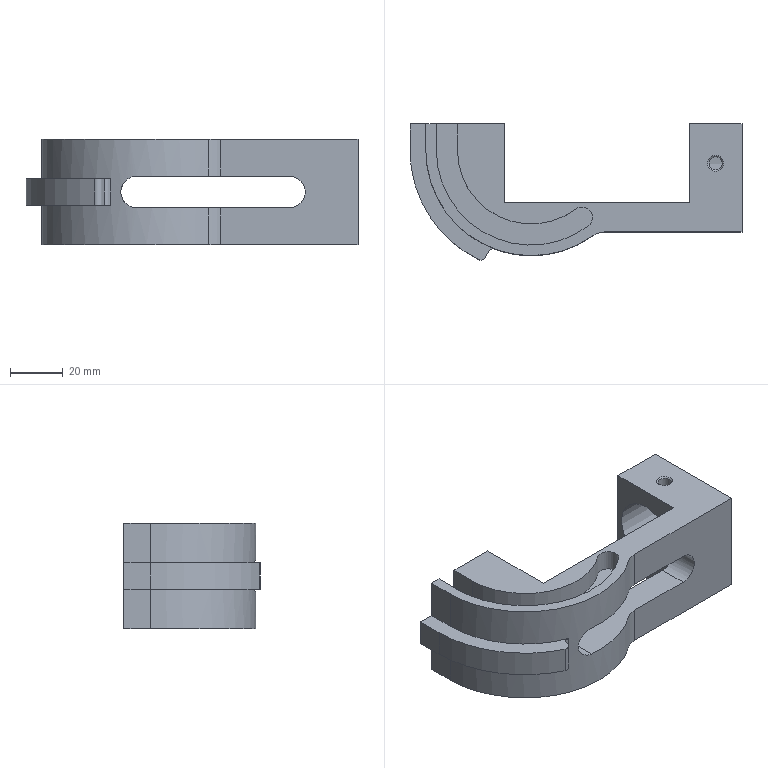Part | NX | features DATUM_CSYS 8, EXTRUDE 7, SKETCH 7, CPROJ 3, BLEND 2, EXTRACT_FACE 2, EXTRACT_STRING 2, HOLE PACKAGE 1, Instance Feature 1, Mirror Feature 1, SIMPLE HOLE 1, SYMBOLIC_THREAD 1 | 1 solid | 41 faces | box 126 x 51.679 x 40 mm | volume 90129 mm3 | plane 24 | cylinder 16 | cone 1 | commonest cylinder face diameters 4 x2 8 x2 12 x2 16 x2 56 x2 72 x2
STEP:
#1=CARTESIAN_POINT('',(-4.,-20.,-6.));
#2=VERTEX_POINT('',#1);
#3=CARTESIAN_POINT('',(-10.,-20.,0.));
#4=VERTEX_POINT('',#3);
#5=CARTESIAN_POINT('',(-4.,-20.,0.));
#6=DIRECTION('',(0.,1.,0.));
#7=DIRECTION('',(1.,0.,0.));
#8=AXIS2_PLACEMENT_3D('',#5,#6,#7);
#9=CIRCLE('',#8,6.);
#10=EDGE_CURVE('',#2,#4,#9,.T.);
#11=ORIENTED_EDGE('',*,*,#10,.F.);
#12=CARTESIAN_POINT('',(54.,-20.,-6.));
#13=VERTEX_POINT('',#12);
#14=CARTESIAN_POINT('',(54.,-20.,-6.));
#15=DIRECTION('',(-1.,0.,0.));
#16=VECTOR('',#15,1000.);
#17=LINE('',#14,#16);
#18=EDGE_CURVE('',#13,#2,#17,.T.);
#19=ORIENTED_EDGE('',*,*,#18,.F.);
#20=CARTESIAN_POINT('',(60.,-20.,0.));
#21=VERTEX_POINT('',#20);
#22=CARTESIAN_POINT('',(54.,-20.,0.));
#23=DIRECTION('',(0.,1.,0.));
#24=DIRECTION('',(1.,0.,0.));
#25=AXIS2_PLACEMENT_3D('',#22,#23,#24);
#26=CIRCLE('',#25,6.);
#27=EDGE_CURVE('',#21,#13,#26,.T.);
#28=ORIENTED_EDGE('',*,*,#27,.F.);
#29=CARTESIAN_POINT('',(60.,-20.,-20.));
#30=VERTEX_POINT('',#29);
#31=CARTESIAN_POINT('',(60.,-20.,45.));
#32=DIRECTION('',(0.,0.,-1.));
#33=VECTOR('',#32,1000.);
#34=LINE('',#31,#33);
#35=EDGE_CURVE('',#30,#21,#34,.F.);
#36=ORIENTED_EDGE('',*,*,#35,.F.);
#37=CARTESIAN_POINT('',(-10.,-20.,-20.));
#38=VERTEX_POINT('',#37);
#39=CARTESIAN_POINT('',(0.,-20.,-20.));
#40=DIRECTION('',(-1.,0.,0.));
#41=VECTOR('',#40,1000.);
#42=LINE('',#39,#41);
#43=EDGE_CURVE('',#30,#38,#42,.T.);
#44=ORIENTED_EDGE('',*,*,#43,.T.);
#45=CARTESIAN_POINT('',(-10.,-20.,45.));
#46=DIRECTION('',(0.,0.,-1.));
#47=VECTOR('',#46,1000.);
#48=LINE('',#45,#47);
#49=EDGE_CURVE('',#38,#4,#48,.F.);
#50=ORIENTED_EDGE('',*,*,#49,.T.);
#51=EDGE_LOOP('',(#11,#19,#28,#36,#44,#50));
#52=FACE_BOUND('',#51,.T.);
#53=CARTESIAN_POINT('',(-10.,-20.,45.));
#54=DIRECTION('',(0.,1.,0.));
#55=DIRECTION('',(0.,0.,1.));
#56=AXIS2_PLACEMENT_3D('',#53,#54,#55);
#57=PLANE('',#56);
#58=ADVANCED_FACE('',(#52),#57,.T.);
#59=CARTESIAN_POINT('',(23.318,-32.5,6.));
#60=VERTEX_POINT('',#59);
#61=CARTESIAN_POINT('',(23.318,-32.5,20.));
#62=VERTEX_POINT('',#61);
#63=CARTESIAN_POINT('',(23.318,-32.5,20.));
#64=DIRECTION('',(0.,0.,-1.));
#65=VECTOR('',#64,1000.);
#66=LINE('',#63,#65);
#67=EDGE_CURVE('',#60,#62,#66,.F.);
#68=ORIENTED_EDGE('',*,*,#67,.F.);
#69=CARTESIAN_POINT('',(27.982,-31.,6.));
#70=VERTEX_POINT('',#69);
#71=CARTESIAN_POINT('',(27.982,-39.,6.));
#72=DIRECTION('',(0.,0.,1.));
#73=DIRECTION('',(1.,0.,0.));
#74=AXIS2_PLACEMENT_3D('',#71,#72,#73);
#75=CIRCLE('',#74,8.);
#76=EDGE_CURVE('',#60,#70,#75,.F.);
#77=ORIENTED_EDGE('',*,*,#76,.T.);
#78=CARTESIAN_POINT('',(27.982,-31.,20.));
#79=VERTEX_POINT('',#78);
#80=CARTESIAN_POINT('',(27.982,-31.,-20.));
#81=DIRECTION('',(0.,0.,1.));
#82=VECTOR('',#81,1000.);
#83=LINE('',#80,#82);
#84=EDGE_CURVE('',#79,#70,#83,.F.);
#85=ORIENTED_EDGE('',*,*,#84,.F.);
#86=CARTESIAN_POINT('',(27.982,-39.,20.));
#87=DIRECTION('',(0.,0.,1.));
#88=DIRECTION('',(1.,0.,0.));
#89=AXIS2_PLACEMENT_3D('',#86,#87,#88);
#90=CIRCLE('',#89,8.);
#91=EDGE_CURVE('',#62,#79,#90,.F.);
#92=ORIENTED_EDGE('',*,*,#91,.F.);
#93=EDGE_LOOP('',(#68,#77,#85,#92));
#94=FACE_BOUND('',#93,.T.);
#95=CARTESIAN_POINT('',(27.982,-39.,20.));
#96=DIRECTION('',(0.,0.,-1.));
#97=DIRECTION('',(-1.,0.,0.));
#98=AXIS2_PLACEMENT_3D('',#95,#96,#97);
#99=CYLINDRICAL_SURFACE('',#98,8.);
#100=ADVANCED_FACE('',(#94),#99,.F.);
#101=CARTESIAN_POINT('',(-40.,0.,5.));
#102=VERTEX_POINT('',#101);
#103=CARTESIAN_POINT('',(-40.,10.,5.));
#104=VERTEX_POINT('',#103);
#105=CARTESIAN_POINT('',(-40.,0.,5.));
#106=DIRECTION('',(0.,1.,0.));
#107=VECTOR('',#106,1000.);
#108=LINE('',#105,#107);
#109=EDGE_CURVE('',#102,#104,#108,.T.);
#110=ORIENTED_EDGE('',*,*,#109,.F.);
#111=CARTESIAN_POINT('',(-40.,0.,20.));
#112=VERTEX_POINT('',#111);
#113=CARTESIAN_POINT('',(-40.,0.,20.));
#114=DIRECTION('',(0.,0.,-1.));
#115=VECTOR('',#114,1000.);
#116=LINE('',#113,#115);
#117=EDGE_CURVE('',#112,#102,#116,.T.);
#118=ORIENTED_EDGE('',*,*,#117,.F.);
#119=CARTESIAN_POINT('',(-40.,10.,20.));
#120=VERTEX_POINT('',#119);
#121=CARTESIAN_POINT('',(-40.,10.,20.));
#122=DIRECTION('',(0.,-1.,0.));
#123=VECTOR('',#122,1000.);
#124=LINE('',#121,#123);
#125=EDGE_CURVE('',#120,#112,#124,.T.);
#126=ORIENTED_EDGE('',*,*,#125,.F.);
#127=CARTESIAN_POINT('',(-40.,10.,20.));
#128=DIRECTION('',(0.,0.,-1.));
#129=VECTOR('',#128,1000.);
#130=LINE('',#127,#129);
#131=EDGE_CURVE('',#120,#104,#130,.T.);
#132=ORIENTED_EDGE('',*,*,#131,.T.);
#133=EDGE_LOOP('',(#110,#118,#126,#132));
#134=FACE_BOUND('',#133,.T.);
#135=CARTESIAN_POINT('',(-40.,10.,20.));
#136=DIRECTION('',(1.,0.,0.));
#137=DIRECTION('',(0.,0.,-1.));
#138=AXIS2_PLACEMENT_3D('',#135,#136,#137);
#139=PLANE('',#138);
#140=ADVANCED_FACE('',(#134),#139,.F.);
#141=CARTESIAN_POINT('',(73.,-5.,20.));
#142=VERTEX_POINT('',#141);
#143=CARTESIAN_POINT('',(70.,-5.,20.));
#144=DIRECTION('',(0.,0.,1.));
#145=DIRECTION('',(1.,0.,0.));
#146=AXIS2_PLACEMENT_3D('',#143,#144,#145);
#147=CIRCLE('',#146,3.);
#148=EDGE_CURVE('',#142,#142,#147,.F.);
#149=ORIENTED_EDGE('',*,*,#148,.T.);
#150=EDGE_LOOP('',(#149));
#151=FACE_BOUND('',#150,.T.);
#152=CARTESIAN_POINT('',(-36.,10.,20.));
#153=VERTEX_POINT('',#152);
#154=CARTESIAN_POINT('',(-36.,0.,20.));
#155=VERTEX_POINT('',#154);
#156=CARTESIAN_POINT('',(-36.,10.,20.));
#157=DIRECTION('',(0.,-1.,0.));
#158=VECTOR('',#157,1000.);
#159=LINE('',#156,#158);
#160=EDGE_CURVE('',#153,#155,#159,.T.);
#161=ORIENTED_EDGE('',*,*,#160,.F.);
#162=CARTESIAN_POINT('',(80.,10.,20.));
#163=DIRECTION('',(-1.,0.,0.));
#164=VECTOR('',#163,1000.);
#165=LINE('',#162,#164);
#166=EDGE_CURVE('',#153,#120,#165,.T.);
#167=ORIENTED_EDGE('',*,*,#166,.T.);
#168=ORIENTED_EDGE('',*,*,#125,.T.);
#169=CARTESIAN_POINT('',(0.,0.,20.));
#170=DIRECTION('',(0.,0.,1.));
#171=DIRECTION('',(1.,0.,0.));
#172=AXIS2_PLACEMENT_3D('',#169,#170,#171);
#173=CIRCLE('',#172,40.);
#174=EDGE_CURVE('',#112,#62,#173,.T.);
#175=ORIENTED_EDGE('',*,*,#174,.T.);
#176=ORIENTED_EDGE('',*,*,#91,.T.);
#177=CARTESIAN_POINT('',(80.,-31.,20.));
#178=VERTEX_POINT('',#177);
#179=CARTESIAN_POINT('',(25.278,-31.,20.));
#180=DIRECTION('',(1.,0.,0.));
#181=VECTOR('',#180,1000.);
#182=LINE('',#179,#181);
#183=EDGE_CURVE('',#79,#178,#182,.T.);
#184=ORIENTED_EDGE('',*,*,#183,.T.);
#185=CARTESIAN_POINT('',(80.,10.,20.));
#186=VERTEX_POINT('',#185);
#187=CARTESIAN_POINT('',(80.,-31.,20.));
#188=DIRECTION('',(0.,1.,0.));
#189=VECTOR('',#188,1000.);
#190=LINE('',#187,#189);
#191=EDGE_CURVE('',#178,#186,#190,.T.);
#192=ORIENTED_EDGE('',*,*,#191,.T.);
#193=CARTESIAN_POINT('',(60.,10.,20.));
#194=VERTEX_POINT('',#193);
#195=CARTESIAN_POINT('',(80.,10.,20.));
#196=DIRECTION('',(-1.,0.,0.));
#197=VECTOR('',#196,1000.);
#198=LINE('',#195,#197);
#199=EDGE_CURVE('',#186,#194,#198,.T.);
#200=ORIENTED_EDGE('',*,*,#199,.T.);
#201=CARTESIAN_POINT('',(60.,-20.,20.));
#202=VERTEX_POINT('',#201);
#203=CARTESIAN_POINT('',(60.,0.,20.));
#204=DIRECTION('',(0.,-1.,0.));
#205=VECTOR('',#204,1000.);
#206=LINE('',#203,#205);
#207=EDGE_CURVE('',#194,#202,#206,.T.);
#208=ORIENTED_EDGE('',*,*,#207,.T.);
#209=CARTESIAN_POINT('',(-10.,-20.,20.));
#210=VERTEX_POINT('',#209);
#211=CARTESIAN_POINT('',(0.,-20.,20.));
#212=DIRECTION('',(-1.,0.,0.));
#213=VECTOR('',#212,1000.);
#214=LINE('',#211,#213);
#215=EDGE_CURVE('',#202,#210,#214,.T.);
#216=ORIENTED_EDGE('',*,*,#215,.T.);
#217=CARTESIAN_POINT('',(-10.,10.,20.));
#218=VERTEX_POINT('',#217);
#219=CARTESIAN_POINT('',(-10.,0.,20.));
#220=DIRECTION('',(0.,1.,0.));
#221=VECTOR('',#220,1000.);
#222=LINE('',#219,#221);
#223=EDGE_CURVE('',#210,#218,#222,.T.);
#224=ORIENTED_EDGE('',*,*,#223,.T.);
#225=CARTESIAN_POINT('',(-28.,10.,20.));
#226=VERTEX_POINT('',#225);
#227=CARTESIAN_POINT('',(80.,10.,20.));
#228=DIRECTION('',(-1.,0.,0.));
#229=VECTOR('',#228,1000.);
#230=LINE('',#227,#229);
#231=EDGE_CURVE('',#218,#226,#230,.T.);
#232=ORIENTED_EDGE('',*,*,#231,.T.);
#233=CARTESIAN_POINT('',(-28.,0.,20.));
#234=VERTEX_POINT('',#233);
#235=CARTESIAN_POINT('',(-28.,0.,20.));
#236=DIRECTION('',(0.,1.,0.));
#237=VECTOR('',#236,1000.);
#238=LINE('',#235,#237);
#239=EDGE_CURVE('',#234,#226,#238,.T.);
#240=ORIENTED_EDGE('',*,*,#239,.F.);
#241=CARTESIAN_POINT('',(16.851,-22.362,20.));
#242=VERTEX_POINT('',#241);
#243=CARTESIAN_POINT('',(0.,0.,20.));
#244=DIRECTION('',(0.,0.,-1.));
#245=DIRECTION('',(1.,0.,0.));
#246=AXIS2_PLACEMENT_3D('',#243,#244,#245);
#247=CIRCLE('',#246,28.);
#248=EDGE_CURVE('',#242,#234,#247,.T.);
#249=ORIENTED_EDGE('',*,*,#248,.F.);
#250=CARTESIAN_POINT('',(21.665,-28.751,20.));
#251=VERTEX_POINT('',#250);
#252=CARTESIAN_POINT('',(19.258,-25.556,20.));
#253=DIRECTION('',(0.,0.,1.));
#254=DIRECTION('',(1.,0.,0.));
#255=AXIS2_PLACEMENT_3D('',#252,#253,#254);
#256=CIRCLE('',#255,4.);
#257=EDGE_CURVE('',#251,#242,#256,.T.);
#258=ORIENTED_EDGE('',*,*,#257,.F.);
#259=CARTESIAN_POINT('',(0.,0.,20.));
#260=DIRECTION('',(0.,0.,1.));
#261=DIRECTION('',(1.,0.,0.));
#262=AXIS2_PLACEMENT_3D('',#259,#260,#261);
#263=CIRCLE('',#262,36.);
#264=EDGE_CURVE('',#155,#251,#263,.T.);
#265=ORIENTED_EDGE('',*,*,#264,.F.);
#266=EDGE_LOOP('',(#161,#167,#168,#175,#176,#184,#192,#200,#208,#216,#224,#232,#240,#249,#258,#265));
#267=FACE_BOUND('',#266,.T.);
#268=CARTESIAN_POINT('',(0.,0.,20.));
#269=DIRECTION('',(0.,0.,1.));
#270=DIRECTION('',(1.,0.,0.));
#271=AXIS2_PLACEMENT_3D('',#268,#269,#270);
#272=PLANE('',#271);
#273=ADVANCED_FACE('',(#151,#267),#272,.T.);
#274=CARTESIAN_POINT('',(60.,10.,-20.));
#275=VERTEX_POINT('',#274);
#276=CARTESIAN_POINT('',(60.,10.,45.));
#277=DIRECTION('',(0.,0.,-1.));
#278=VECTOR('',#277,1000.);
#279=LINE('',#276,#278);
#280=EDGE_CURVE('',#194,#275,#279,.T.);
#281=ORIENTED_EDGE('',*,*,#280,.F.);
#282=ORIENTED_EDGE('',*,*,#199,.F.);
#283=CARTESIAN_POINT('',(80.,10.,-20.));
#284=VERTEX_POINT('',#283);
#285=CARTESIAN_POINT('',(80.,10.,20.));
#286=DIRECTION('',(0.,0.,-1.));
#287=VECTOR('',#286,1000.);
#288=LINE('',#285,#287);
#289=EDGE_CURVE('',#186,#284,#288,.T.);
#290=ORIENTED_EDGE('',*,*,#289,.T.);
#291=CARTESIAN_POINT('',(80.,10.,-20.));
#292=DIRECTION('',(-1.,0.,0.));
#293=VECTOR('',#292,1000.);
#294=LINE('',#291,#293);
#295=EDGE_CURVE('',#284,#275,#294,.T.);
#296=ORIENTED_EDGE('',*,*,#295,.T.);
#297=EDGE_LOOP('',(#281,#282,#290,#296));
#298=FACE_BOUND('',#297,.T.);
#299=CARTESIAN_POINT('',(80.,10.,20.));
#300=DIRECTION('',(0.,-1.,0.));
#301=DIRECTION('',(1.,0.,0.));
#302=AXIS2_PLACEMENT_3D('',#299,#300,#301);
#303=PLANE('',#302);
#304=ADVANCED_FACE('',(#298),#303,.F.);
#305=CARTESIAN_POINT('',(-36.,10.,-20.));
#306=VERTEX_POINT('',#305);
#307=CARTESIAN_POINT('',(-40.,10.,-20.));
#308=VERTEX_POINT('',#307);
#309=CARTESIAN_POINT('',(80.,10.,-20.));
#310=DIRECTION('',(-1.,0.,0.));
#311=VECTOR('',#310,1000.);
#312=LINE('',#309,#311);
#313=EDGE_CURVE('',#306,#308,#312,.T.);
#314=ORIENTED_EDGE('',*,*,#313,.F.);
#315=CARTESIAN_POINT('',(-36.,0.,-20.));
#316=VERTEX_POINT('',#315);
#317=CARTESIAN_POINT('',(-36.,10.,-20.));
#318=DIRECTION('',(0.,-1.,0.));
#319=VECTOR('',#318,1000.);
#320=LINE('',#317,#319);
#321=EDGE_CURVE('',#306,#316,#320,.T.);
#322=ORIENTED_EDGE('',*,*,#321,.T.);
#323=CARTESIAN_POINT('',(21.665,-28.751,-20.));
#324=VERTEX_POINT('',#323);
#325=CARTESIAN_POINT('',(0.,0.,-20.));
#326=DIRECTION('',(0.,0.,1.));
#327=DIRECTION('',(1.,0.,0.));
#328=AXIS2_PLACEMENT_3D('',#325,#326,#327);
#329=CIRCLE('',#328,36.);
#330=EDGE_CURVE('',#316,#324,#329,.T.);
#331=ORIENTED_EDGE('',*,*,#330,.T.);
#332=CARTESIAN_POINT('',(16.851,-22.362,-20.));
#333=VERTEX_POINT('',#332);
#334=CARTESIAN_POINT('',(19.258,-25.556,-20.));
#335=DIRECTION('',(0.,0.,1.));
#336=DIRECTION('',(1.,0.,0.));
#337=AXIS2_PLACEMENT_3D('',#334,#335,#336);
#338=CIRCLE('',#337,4.);
#339=EDGE_CURVE('',#324,#333,#338,.T.);
#340=ORIENTED_EDGE('',*,*,#339,.T.);
#341=CARTESIAN_POINT('',(-28.,0.,-20.));
#342=VERTEX_POINT('',#341);
#343=CARTESIAN_POINT('',(0.,0.,-20.));
#344=DIRECTION('',(0.,0.,-1.));
#345=DIRECTION('',(1.,0.,0.));
#346=AXIS2_PLACEMENT_3D('',#343,#344,#345);
#347=CIRCLE('',#346,28.);
#348=EDGE_CURVE('',#333,#342,#347,.T.);
#349=ORIENTED_EDGE('',*,*,#348,.T.);
#350=CARTESIAN_POINT('',(-28.,10.,-20.));
#351=VERTEX_POINT('',#350);
#352=CARTESIAN_POINT('',(-28.,0.,-20.));
#353=DIRECTION('',(0.,1.,0.));
#354=VECTOR('',#353,1000.);
#355=LINE('',#352,#354);
#356=EDGE_CURVE('',#342,#351,#355,.T.);
#357=ORIENTED_EDGE('',*,*,#356,.T.);
#358=CARTESIAN_POINT('',(-10.,10.,-20.));
#359=VERTEX_POINT('',#358);
#360=CARTESIAN_POINT('',(80.,10.,-20.));
#361=DIRECTION('',(-1.,0.,0.));
#362=VECTOR('',#361,1000.);
#363=LINE('',#360,#362);
#364=EDGE_CURVE('',#359,#351,#363,.T.);
#365=ORIENTED_EDGE('',*,*,#364,.F.);
#366=CARTESIAN_POINT('',(-10.,0.,-20.));
#367=DIRECTION('',(0.,1.,0.));
#368=VECTOR('',#367,1000.);
#369=LINE('',#366,#368);
#370=EDGE_CURVE('',#38,#359,#369,.T.);
#371=ORIENTED_EDGE('',*,*,#370,.F.);
#372=ORIENTED_EDGE('',*,*,#43,.F.);
#373=CARTESIAN_POINT('',(60.,0.,-20.));
#374=DIRECTION('',(0.,-1.,0.));
#375=VECTOR('',#374,1000.);
#376=LINE('',#373,#375);
#377=EDGE_CURVE('',#275,#30,#376,.T.);
#378=ORIENTED_EDGE('',*,*,#377,.F.);
#379=ORIENTED_EDGE('',*,*,#295,.F.);
#380=CARTESIAN_POINT('',(80.,-31.,-20.));
#381=VERTEX_POINT('',#380);
#382=CARTESIAN_POINT('',(80.,-31.,-20.));
#383=DIRECTION('',(0.,1.,0.));
#384=VECTOR('',#383,1000.);
#385=LINE('',#382,#384);
#386=EDGE_CURVE('',#381,#284,#385,.T.);
#387=ORIENTED_EDGE('',*,*,#386,.F.);
#388=CARTESIAN_POINT('',(27.982,-31.,-20.));
#389=VERTEX_POINT('',#388);
#390=CARTESIAN_POINT('',(25.278,-31.,-20.));
#391=DIRECTION('',(1.,0.,0.));
#392=VECTOR('',#391,1000.);
#393=LINE('',#390,#392);
#394=EDGE_CURVE('',#389,#381,#393,.T.);
#395=ORIENTED_EDGE('',*,*,#394,.F.);
#396=CARTESIAN_POINT('',(23.318,-32.5,-20.));
#397=VERTEX_POINT('',#396);
#398=CARTESIAN_POINT('',(27.982,-39.,-20.));
#399=DIRECTION('',(0.,0.,1.));
#400=DIRECTION('',(1.,0.,0.));
#401=AXIS2_PLACEMENT_3D('',#398,#399,#400);
#402=CIRCLE('',#401,8.);
#403=EDGE_CURVE('',#389,#397,#402,.T.);
#404=ORIENTED_EDGE('',*,*,#403,.T.);
#405=CARTESIAN_POINT('',(-40.,0.,-20.));
#406=VERTEX_POINT('',#405);
#407=CARTESIAN_POINT('',(0.,0.,-20.));
#408=DIRECTION('',(0.,0.,1.));
#409=DIRECTION('',(1.,0.,0.));
#410=AXIS2_PLACEMENT_3D('',#407,#408,#409);
#411=CIRCLE('',#410,40.);
#412=EDGE_CURVE('',#406,#397,#411,.T.);
#413=ORIENTED_EDGE('',*,*,#412,.F.);
#414=CARTESIAN_POINT('',(-40.,10.,-20.));
#415=DIRECTION('',(0.,-1.,0.));
#416=VECTOR('',#415,1000.);
#417=LINE('',#414,#416);
#418=EDGE_CURVE('',#308,#406,#417,.T.);
#419=ORIENTED_EDGE('',*,*,#418,.F.);
#420=EDGE_LOOP('',(#314,#322,#331,#340,#349,#357,#365,#371,#372,#378,#379,#387,#395,#404,#413,#419));
#421=FACE_BOUND('',#420,.T.);
#422=CARTESIAN_POINT('',(0.,0.,-20.));
#423=DIRECTION('',(0.,0.,1.));
#424=DIRECTION('',(1.,0.,0.));
#425=AXIS2_PLACEMENT_3D('',#422,#423,#424);
#426=PLANE('',#425);
#427=ADVANCED_FACE('',(#421),#426,.F.);
#428=CARTESIAN_POINT('',(-13.858,-37.523,5.));
#429=VERTEX_POINT('',#428);
#430=CARTESIAN_POINT('',(-13.858,-37.523,-5.));
#431=VERTEX_POINT('',#430);
#432=CARTESIAN_POINT('',(-13.858,-37.523,20.));
#433=DIRECTION('',(0.,0.,-1.));
#434=VECTOR('',#433,1000.);
#435=LINE('',#432,#434);
#436=EDGE_CURVE('',#429,#431,#435,.T.);
#437=ORIENTED_EDGE('',*,*,#436,.T.);
#438=CARTESIAN_POINT('',(-40.,0.,-5.));
#439=VERTEX_POINT('',#438);
#440=CARTESIAN_POINT('',(0.,0.,-5.));
#441=DIRECTION('',(0.,0.,-1.));
#442=DIRECTION('',(1.,0.,0.));
#443=AXIS2_PLACEMENT_3D('',#440,#441,#442);
#444=CIRCLE('',#443,40.);
#445=EDGE_CURVE('',#431,#439,#444,.T.);
#446=ORIENTED_EDGE('',*,*,#445,.T.);
#447=CARTESIAN_POINT('',(-40.,0.,20.));
#448=DIRECTION('',(0.,0.,-1.));
#449=VECTOR('',#448,1000.);
#450=LINE('',#447,#449);
#451=EDGE_CURVE('',#439,#406,#450,.T.);
#452=ORIENTED_EDGE('',*,*,#451,.T.);
#453=ORIENTED_EDGE('',*,*,#412,.T.);
#454=CARTESIAN_POINT('',(23.318,-32.5,-6.));
#455=VERTEX_POINT('',#454);
#456=CARTESIAN_POINT('',(23.318,-32.5,20.));
#457=DIRECTION('',(0.,0.,-1.));
#458=VECTOR('',#457,1000.);
#459=LINE('',#456,#458);
#460=EDGE_CURVE('',#397,#455,#459,.F.);
#461=ORIENTED_EDGE('',*,*,#460,.T.);
#462=CARTESIAN_POINT('',(-4.,-39.799,-6.));
#463=VERTEX_POINT('',#462);
#464=CARTESIAN_POINT('',(0.,0.,-6.));
#465=DIRECTION('',(0.,0.,-1.));
#466=DIRECTION('',(-1.,0.,0.));
#467=AXIS2_PLACEMENT_3D('',#464,#465,#466);
#468=CIRCLE('',#467,40.);
#469=EDGE_CURVE('',#455,#463,#468,.T.);
#470=ORIENTED_EDGE('',*,*,#469,.T.);
#471=CARTESIAN_POINT('',(-4.,-39.799,6.));
#472=VERTEX_POINT('',#471);
#473=CARTESIAN_POINT('',(-4.,-39.799,-6.));
#474=CARTESIAN_POINT('',(-5.589,-39.64,-6.));
#475=CARTESIAN_POINT('',(-8.674,-39.102,-4.714));
#476=CARTESIAN_POINT('',(-10.662,-38.544,-0.008833));
#477=CARTESIAN_POINT('',(-8.679,-39.101,4.714));
#478=CARTESIAN_POINT('',(-5.589,-39.64,6.));
#479=CARTESIAN_POINT('',(-4.,-39.799,6.));
#480=B_SPLINE_CURVE_WITH_KNOTS('',3,(#473,#474,#475,#476,#477,#478,#479),.UNSPECIFIED.,.F.,.F.,(4,1,1,1,4),(0.,0.004722,0.009444,0.01417,0.01889),.UNSPECIFIED.);
#481=EDGE_CURVE('',#463,#472,#480,.T.);
#482=ORIENTED_EDGE('',*,*,#481,.T.);
#483=CARTESIAN_POINT('',(0.,0.,6.));
#484=DIRECTION('',(0.,0.,1.));
#485=DIRECTION('',(1.,0.,0.));
#486=AXIS2_PLACEMENT_3D('',#483,#484,#485);
#487=CIRCLE('',#486,40.);
#488=EDGE_CURVE('',#472,#60,#487,.T.);
#489=ORIENTED_EDGE('',*,*,#488,.T.);
#490=ORIENTED_EDGE('',*,*,#67,.T.);
#491=ORIENTED_EDGE('',*,*,#174,.F.);
#492=ORIENTED_EDGE('',*,*,#117,.T.);
#493=CARTESIAN_POINT('',(0.,0.,5.));
#494=DIRECTION('',(0.,0.,-1.));
#495=DIRECTION('',(1.,0.,0.));
#496=AXIS2_PLACEMENT_3D('',#493,#494,#495);
#497=CIRCLE('',#496,40.);
#498=EDGE_CURVE('',#429,#102,#497,.T.);
#499=ORIENTED_EDGE('',*,*,#498,.F.);
#500=EDGE_LOOP('',(#437,#446,#452,#453,#461,#470,#482,#489,#490,#491,#492,#499));
#501=FACE_BOUND('',#500,.T.);
#502=CARTESIAN_POINT('',(0.,0.,20.));
#503=DIRECTION('',(0.,0.,-1.));
#504=DIRECTION('',(-1.,0.,0.));
#505=AXIS2_PLACEMENT_3D('',#502,#503,#504);
#506=CYLINDRICAL_SURFACE('',#505,40.);
#507=ADVANCED_FACE('',(#501),#506,.T.);
#508=ORIENTED_EDGE('',*,*,#84,.T.);
#509=CARTESIAN_POINT('',(54.,-31.,6.));
#510=VERTEX_POINT('',#509);
#511=CARTESIAN_POINT('',(25.278,-31.,6.));
#512=DIRECTION('',(1.,0.,0.));
#513=VECTOR('',#512,1000.);
#514=LINE('',#511,#513);
#515=EDGE_CURVE('',#70,#510,#514,.T.);
#516=ORIENTED_EDGE('',*,*,#515,.T.);
#517=CARTESIAN_POINT('',(54.,-31.,-6.));
#518=VERTEX_POINT('',#517);
#519=CARTESIAN_POINT('',(54.,-31.,0.));
#520=DIRECTION('',(0.,1.,0.));
#521=DIRECTION('',(-1.,0.,0.));
#522=AXIS2_PLACEMENT_3D('',#519,#520,#521);
#523=CIRCLE('',#522,6.);
#524=EDGE_CURVE('',#510,#518,#523,.T.);
#525=ORIENTED_EDGE('',*,*,#524,.T.);
#526=CARTESIAN_POINT('',(27.982,-31.,-6.));
#527=VERTEX_POINT('',#526);
#528=CARTESIAN_POINT('',(25.278,-31.,-6.));
#529=DIRECTION('',(-1.,0.,0.));
#530=VECTOR('',#529,1000.);
#531=LINE('',#528,#530);
#532=EDGE_CURVE('',#518,#527,#531,.T.);
#533=ORIENTED_EDGE('',*,*,#532,.T.);
#534=CARTESIAN_POINT('',(27.982,-31.,-20.));
#535=DIRECTION('',(0.,0.,1.));
#536=VECTOR('',#535,1000.);
#537=LINE('',#534,#536);
#538=EDGE_CURVE('',#527,#389,#537,.F.);
#539=ORIENTED_EDGE('',*,*,#538,.T.);
#540=ORIENTED_EDGE('',*,*,#394,.T.);
#541=CARTESIAN_POINT('',(80.,-31.,20.));
#542=DIRECTION('',(0.,0.,-1.));
#543=VECTOR('',#542,1000.);
#544=LINE('',#541,#543);
#545=EDGE_CURVE('',#178,#381,#544,.T.);
#546=ORIENTED_EDGE('',*,*,#545,.F.);
#547=ORIENTED_EDGE('',*,*,#183,.F.);
#548=EDGE_LOOP('',(#508,#516,#525,#533,#539,#540,#546,#547));
#549=FACE_BOUND('',#548,.T.);
#550=CARTESIAN_POINT('',(25.278,-31.,20.));
#551=DIRECTION('',(0.,1.,0.));
#552=DIRECTION('',(-1.,0.,0.));
#553=AXIS2_PLACEMENT_3D('',#550,#551,#552);
#554=PLANE('',#553);
#555=ADVANCED_FACE('',(#549),#554,.F.);
#556=CARTESIAN_POINT('',(80.,-5.,-13.));
#557=VERTEX_POINT('',#556);
#558=CARTESIAN_POINT('',(80.,-5.,0.));
#559=DIRECTION('',(1.,0.,0.));
#560=DIRECTION('',(0.,0.,-1.));
#561=AXIS2_PLACEMENT_3D('',#558,#559,#560);
#562=CIRCLE('',#561,13.);
#563=EDGE_CURVE('',#557,#557,#562,.T.);
#564=ORIENTED_EDGE('',*,*,#563,.F.);
#565=EDGE_LOOP('',(#564));
#566=FACE_BOUND('',#565,.T.);
#567=ORIENTED_EDGE('',*,*,#386,.T.);
#568=ORIENTED_EDGE('',*,*,#289,.F.);
#569=ORIENTED_EDGE('',*,*,#191,.F.);
#570=ORIENTED_EDGE('',*,*,#545,.T.);
#571=EDGE_LOOP('',(#567,#568,#569,#570));
#572=FACE_BOUND('',#571,.T.);
#573=CARTESIAN_POINT('',(80.,-31.,20.));
#574=DIRECTION('',(-1.,0.,0.));
#575=DIRECTION('',(0.,0.,1.));
#576=AXIS2_PLACEMENT_3D('',#573,#574,#575);
#577=PLANE('',#576);
#578=ADVANCED_FACE('',(#566,#572),#577,.F.);
#579=CARTESIAN_POINT('',(-28.,10.,-12.));
#580=VERTEX_POINT('',#579);
#581=CARTESIAN_POINT('',(-36.,10.,-12.));
#582=VERTEX_POINT('',#581);
#583=CARTESIAN_POINT('',(-28.,10.,-12.));
#584=DIRECTION('',(-1.,0.,0.));
#585=VECTOR('',#584,1000.);
#586=LINE('',#583,#585);
#587=EDGE_CURVE('',#580,#582,#586,.T.);
#588=ORIENTED_EDGE('',*,*,#587,.T.);
#589=CARTESIAN_POINT('',(-36.,10.,-12.));
#590=DIRECTION('',(0.,0.,-1.));
#591=VECTOR('',#590,1000.);
#592=LINE('',#589,#591);
#593=EDGE_CURVE('',#582,#306,#592,.T.);
#594=ORIENTED_EDGE('',*,*,#593,.T.);
#595=ORIENTED_EDGE('',*,*,#313,.T.);
#596=CARTESIAN_POINT('',(-40.,10.,-5.));
#597=VERTEX_POINT('',#596);
#598=CARTESIAN_POINT('',(-40.,10.,20.));
#599=DIRECTION('',(0.,0.,-1.));
#600=VECTOR('',#599,1000.);
#601=LINE('',#598,#600);
#602=EDGE_CURVE('',#597,#308,#601,.T.);
#603=ORIENTED_EDGE('',*,*,#602,.F.);
#604=CARTESIAN_POINT('',(-46.,10.,-5.));
#605=VERTEX_POINT('',#604);
#606=CARTESIAN_POINT('',(-40.,10.,-5.));
#607=DIRECTION('',(-1.,0.,0.));
#608=VECTOR('',#607,1000.);
#609=LINE('',#606,#608);
#610=EDGE_CURVE('',#597,#605,#609,.T.);
#611=ORIENTED_EDGE('',*,*,#610,.T.);
#612=CARTESIAN_POINT('',(-46.,10.,5.));
#613=VERTEX_POINT('',#612);
#614=CARTESIAN_POINT('',(-46.,10.,5.));
#615=DIRECTION('',(0.,0.,-1.));
#616=VECTOR('',#615,1000.);
#617=LINE('',#614,#616);
#618=EDGE_CURVE('',#613,#605,#617,.T.);
#619=ORIENTED_EDGE('',*,*,#618,.F.);
#620=CARTESIAN_POINT('',(-40.,10.,5.));
#621=DIRECTION('',(-1.,0.,0.));
#622=VECTOR('',#621,1000.);
#623=LINE('',#620,#622);
#624=EDGE_CURVE('',#104,#613,#623,.T.);
#625=ORIENTED_EDGE('',*,*,#624,.F.);
#626=ORIENTED_EDGE('',*,*,#131,.F.);
#627=ORIENTED_EDGE('',*,*,#166,.F.);
#628=CARTESIAN_POINT('',(-36.,10.,12.));
#629=VERTEX_POINT('',#628);
#630=CARTESIAN_POINT('',(-36.,10.,12.));
#631=DIRECTION('',(0.,0.,1.));
#632=VECTOR('',#631,1000.);
#633=LINE('',#630,#632);
#634=EDGE_CURVE('',#629,#153,#633,.T.);
#635=ORIENTED_EDGE('',*,*,#634,.F.);
#636=CARTESIAN_POINT('',(-28.,10.,12.));
#637=VERTEX_POINT('',#636);
#638=CARTESIAN_POINT('',(-28.,10.,12.));
#639=DIRECTION('',(-1.,0.,0.));
#640=VECTOR('',#639,1000.);
#641=LINE('',#638,#640);
#642=EDGE_CURVE('',#637,#629,#641,.T.);
#643=ORIENTED_EDGE('',*,*,#642,.F.);
#644=CARTESIAN_POINT('',(-28.,10.,12.));
#645=DIRECTION('',(0.,0.,1.));
#646=VECTOR('',#645,1000.);
#647=LINE('',#644,#646);
#648=EDGE_CURVE('',#637,#226,#647,.T.);
#649=ORIENTED_EDGE('',*,*,#648,.T.);
#650=ORIENTED_EDGE('',*,*,#231,.F.);
#651=CARTESIAN_POINT('',(-10.,10.,45.));
#652=DIRECTION('',(0.,0.,-1.));
#653=VECTOR('',#652,1000.);
#654=LINE('',#651,#653);
#655=EDGE_CURVE('',#218,#359,#654,.T.);
#656=ORIENTED_EDGE('',*,*,#655,.T.);
#657=ORIENTED_EDGE('',*,*,#364,.T.);
#658=CARTESIAN_POINT('',(-28.,10.,-12.));
#659=DIRECTION('',(0.,0.,-1.));
#660=VECTOR('',#659,1000.);
#661=LINE('',#658,#660);
#662=EDGE_CURVE('',#580,#351,#661,.T.);
#663=ORIENTED_EDGE('',*,*,#662,.F.);
#664=EDGE_LOOP('',(#588,#594,#595,#603,#611,#619,#625,#626,#627,#635,#643,#649,#650,#656,#657,#663));
#665=FACE_BOUND('',#664,.T.);
#666=CARTESIAN_POINT('',(80.,10.,20.));
#667=DIRECTION('',(0.,-1.,0.));
#668=DIRECTION('',(1.,0.,0.));
#669=AXIS2_PLACEMENT_3D('',#666,#667,#668);
#670=PLANE('',#669);
#671=ADVANCED_FACE('',(#665),#670,.F.);
#672=ORIENTED_EDGE('',*,*,#451,.F.);
#673=CARTESIAN_POINT('',(-40.,0.,-5.));
#674=DIRECTION('',(0.,1.,0.));
#675=VECTOR('',#674,1000.);
#676=LINE('',#673,#675);
#677=EDGE_CURVE('',#439,#597,#676,.T.);
#678=ORIENTED_EDGE('',*,*,#677,.T.);
#679=ORIENTED_EDGE('',*,*,#602,.T.);
#680=ORIENTED_EDGE('',*,*,#418,.T.);
#681=EDGE_LOOP('',(#672,#678,#679,#680));
#682=FACE_BOUND('',#681,.T.);
#683=CARTESIAN_POINT('',(-40.,10.,20.));
#684=DIRECTION('',(1.,0.,0.));
#685=DIRECTION('',(0.,0.,-1.));
#686=AXIS2_PLACEMENT_3D('',#683,#684,#685);
#687=PLANE('',#686);
#688=ADVANCED_FACE('',(#682),#687,.F.);
#689=ORIENTED_EDGE('',*,*,#49,.F.);
#690=ORIENTED_EDGE('',*,*,#370,.T.);
#691=ORIENTED_EDGE('',*,*,#655,.F.);
#692=ORIENTED_EDGE('',*,*,#223,.F.);
#693=CARTESIAN_POINT('',(-10.,-20.,45.));
#694=DIRECTION('',(0.,0.,-1.));
#695=VECTOR('',#694,1000.);
#696=LINE('',#693,#695);
#697=EDGE_CURVE('',#4,#210,#696,.F.);
#698=ORIENTED_EDGE('',*,*,#697,.F.);
#699=EDGE_LOOP('',(#689,#690,#691,#692,#698));
#700=FACE_BOUND('',#699,.T.);
#701=CARTESIAN_POINT('',(-10.,10.,45.));
#702=DIRECTION('',(1.,0.,0.));
#703=DIRECTION('',(0.,0.,-1.));
#704=AXIS2_PLACEMENT_3D('',#701,#702,#703);
#705=PLANE('',#704);
#706=ADVANCED_FACE('',(#700),#705,.T.);
#707=CARTESIAN_POINT('',(-4.,-20.,6.));
#708=VERTEX_POINT('',#707);
#709=CARTESIAN_POINT('',(-4.,-20.,0.));
#710=DIRECTION('',(0.,1.,0.));
#711=DIRECTION('',(1.,0.,0.));
#712=AXIS2_PLACEMENT_3D('',#709,#710,#711);
#713=CIRCLE('',#712,6.);
#714=EDGE_CURVE('',#4,#708,#713,.T.);
#715=ORIENTED_EDGE('',*,*,#714,.F.);
#716=ORIENTED_EDGE('',*,*,#697,.T.);
#717=ORIENTED_EDGE('',*,*,#215,.F.);
#718=CARTESIAN_POINT('',(60.,-20.,45.));
#719=DIRECTION('',(0.,0.,-1.));
#720=VECTOR('',#719,1000.);
#721=LINE('',#718,#720);
#722=EDGE_CURVE('',#21,#202,#721,.F.);
#723=ORIENTED_EDGE('',*,*,#722,.F.);
#724=CARTESIAN_POINT('',(54.,-20.,6.));
#725=VERTEX_POINT('',#724);
#726=CARTESIAN_POINT('',(54.,-20.,0.));
#727=DIRECTION('',(0.,1.,0.));
#728=DIRECTION('',(1.,0.,0.));
#729=AXIS2_PLACEMENT_3D('',#726,#727,#728);
#730=CIRCLE('',#729,6.);
#731=EDGE_CURVE('',#725,#21,#730,.T.);
#732=ORIENTED_EDGE('',*,*,#731,.F.);
#733=CARTESIAN_POINT('',(-4.,-20.,6.));
#734=DIRECTION('',(1.,0.,0.));
#735=VECTOR('',#734,1000.);
#736=LINE('',#733,#735);
#737=EDGE_CURVE('',#708,#725,#736,.T.);
#738=ORIENTED_EDGE('',*,*,#737,.F.);
#739=EDGE_LOOP('',(#715,#716,#717,#723,#732,#738));
#740=FACE_BOUND('',#739,.T.);
#741=CARTESIAN_POINT('',(-10.,-20.,45.));
#742=DIRECTION('',(0.,1.,0.));
#743=DIRECTION('',(0.,0.,1.));
#744=AXIS2_PLACEMENT_3D('',#741,#742,#743);
#745=PLANE('',#744);
#746=ADVANCED_FACE('',(#740),#745,.T.);
#747=CARTESIAN_POINT('',(60.,-5.,13.));
#748=VERTEX_POINT('',#747);
#749=CARTESIAN_POINT('',(60.,-5.,0.));
#750=DIRECTION('',(-1.,0.,0.));
#751=DIRECTION('',(0.,0.,1.));
#752=AXIS2_PLACEMENT_3D('',#749,#750,#751);
#753=CIRCLE('',#752,13.);
#754=EDGE_CURVE('',#748,#748,#753,.T.);
#755=ORIENTED_EDGE('',*,*,#754,.F.);
#756=EDGE_LOOP('',(#755));
#757=FACE_BOUND('',#756,.T.);
#758=ORIENTED_EDGE('',*,*,#280,.T.);
#759=ORIENTED_EDGE('',*,*,#377,.T.);
#760=ORIENTED_EDGE('',*,*,#35,.T.);
#761=ORIENTED_EDGE('',*,*,#722,.T.);
#762=ORIENTED_EDGE('',*,*,#207,.F.);
#763=EDGE_LOOP('',(#758,#759,#760,#761,#762));
#764=FACE_BOUND('',#763,.T.);
#765=CARTESIAN_POINT('',(60.,-20.,45.));
#766=DIRECTION('',(-1.,0.,0.));
#767=DIRECTION('',(0.,0.,1.));
#768=AXIS2_PLACEMENT_3D('',#765,#766,#767);
#769=PLANE('',#768);
#770=ADVANCED_FACE('',(#757,#764),#769,.T.);
#771=ORIENTED_EDGE('',*,*,#160,.T.);
#772=CARTESIAN_POINT('',(-36.,0.,12.));
#773=VERTEX_POINT('',#772);
#774=CARTESIAN_POINT('',(-36.,0.,12.));
#775=DIRECTION('',(0.,0.,1.));
#776=VECTOR('',#775,1000.);
#777=LINE('',#774,#776);
#778=EDGE_CURVE('',#155,#773,#777,.F.);
#779=ORIENTED_EDGE('',*,*,#778,.T.);
#780=CARTESIAN_POINT('',(-36.,10.,12.));
#781=DIRECTION('',(0.,-1.,0.));
#782=VECTOR('',#781,1000.);
#783=LINE('',#780,#782);
#784=EDGE_CURVE('',#773,#629,#783,.F.);
#785=ORIENTED_EDGE('',*,*,#784,.T.);
#786=ORIENTED_EDGE('',*,*,#634,.T.);
#787=EDGE_LOOP('',(#771,#779,#785,#786));
#788=FACE_BOUND('',#787,.T.);
#789=CARTESIAN_POINT('',(-36.,10.,12.));
#790=DIRECTION('',(-1.,0.,0.));
#791=DIRECTION('',(0.,0.,1.));
#792=AXIS2_PLACEMENT_3D('',#789,#790,#791);
#793=PLANE('',#792);
#794=ADVANCED_FACE('',(#788),#793,.F.);
#795=ORIENTED_EDGE('',*,*,#264,.T.);
#796=CARTESIAN_POINT('',(21.665,-28.751,12.));
#797=VERTEX_POINT('',#796);
#798=CARTESIAN_POINT('',(21.665,-28.751,12.));
#799=DIRECTION('',(0.,0.,1.));
#800=VECTOR('',#799,1000.);
#801=LINE('',#798,#800);
#802=EDGE_CURVE('',#251,#797,#801,.F.);
#803=ORIENTED_EDGE('',*,*,#802,.T.);
#804=CARTESIAN_POINT('',(0.,0.,12.));
#805=DIRECTION('',(0.,0.,1.));
#806=DIRECTION('',(1.,0.,0.));
#807=AXIS2_PLACEMENT_3D('',#804,#805,#806);
#808=CIRCLE('',#807,36.);
#809=EDGE_CURVE('',#797,#773,#808,.F.);
#810=ORIENTED_EDGE('',*,*,#809,.T.);
#811=ORIENTED_EDGE('',*,*,#778,.F.);
#812=EDGE_LOOP('',(#795,#803,#810,#811));
#813=FACE_BOUND('',#812,.T.);
#814=CARTESIAN_POINT('',(0.,0.,12.));
#815=DIRECTION('',(0.,0.,1.));
#816=DIRECTION('',(1.,0.,0.));
#817=AXIS2_PLACEMENT_3D('',#814,#815,#816);
#818=CYLINDRICAL_SURFACE('',#817,36.);
#819=ADVANCED_FACE('',(#813),#818,.F.);
#820=ORIENTED_EDGE('',*,*,#257,.T.);
#821=CARTESIAN_POINT('',(16.851,-22.362,12.));
#822=VERTEX_POINT('',#821);
#823=CARTESIAN_POINT('',(16.851,-22.362,12.));
#824=DIRECTION('',(0.,0.,1.));
#825=VECTOR('',#824,1000.);
#826=LINE('',#823,#825);
#827=EDGE_CURVE('',#242,#822,#826,.F.);
#828=ORIENTED_EDGE('',*,*,#827,.T.);
#829=CARTESIAN_POINT('',(19.258,-25.556,12.));
#830=DIRECTION('',(0.,0.,1.));
#831=DIRECTION('',(1.,0.,0.));
#832=AXIS2_PLACEMENT_3D('',#829,#830,#831);
#833=CIRCLE('',#832,4.);
#834=EDGE_CURVE('',#822,#797,#833,.F.);
#835=ORIENTED_EDGE('',*,*,#834,.T.);
#836=ORIENTED_EDGE('',*,*,#802,.F.);
#837=EDGE_LOOP('',(#820,#828,#835,#836));
#838=FACE_BOUND('',#837,.T.);
#839=CARTESIAN_POINT('',(19.258,-25.556,12.));
#840=DIRECTION('',(0.,0.,1.));
#841=DIRECTION('',(1.,0.,0.));
#842=AXIS2_PLACEMENT_3D('',#839,#840,#841);
#843=CYLINDRICAL_SURFACE('',#842,4.);
#844=ADVANCED_FACE('',(#838),#843,.F.);
#845=ORIENTED_EDGE('',*,*,#248,.T.);
#846=CARTESIAN_POINT('',(-28.,0.,12.));
#847=VERTEX_POINT('',#846);
#848=CARTESIAN_POINT('',(-28.,0.,12.));
#849=DIRECTION('',(0.,0.,1.));
#850=VECTOR('',#849,1000.);
#851=LINE('',#848,#850);
#852=EDGE_CURVE('',#234,#847,#851,.F.);
#853=ORIENTED_EDGE('',*,*,#852,.T.);
#854=CARTESIAN_POINT('',(0.,0.,12.));
#855=DIRECTION('',(0.,0.,-1.));
#856=DIRECTION('',(1.,0.,0.));
#857=AXIS2_PLACEMENT_3D('',#854,#855,#856);
#858=CIRCLE('',#857,28.);
#859=EDGE_CURVE('',#847,#822,#858,.F.);
#860=ORIENTED_EDGE('',*,*,#859,.T.);
#861=ORIENTED_EDGE('',*,*,#827,.F.);
#862=EDGE_LOOP('',(#845,#853,#860,#861));
#863=FACE_BOUND('',#862,.T.);
#864=CARTESIAN_POINT('',(0.,0.,12.));
#865=DIRECTION('',(0.,0.,1.));
#866=DIRECTION('',(1.,0.,0.));
#867=AXIS2_PLACEMENT_3D('',#864,#865,#866);
#868=CYLINDRICAL_SURFACE('',#867,28.);
#869=ADVANCED_FACE('',(#863),#868,.T.);
#870=ORIENTED_EDGE('',*,*,#239,.T.);
#871=ORIENTED_EDGE('',*,*,#648,.F.);
#872=CARTESIAN_POINT('',(-28.,0.,12.));
#873=DIRECTION('',(0.,1.,0.));
#874=VECTOR('',#873,1000.);
#875=LINE('',#872,#874);
#876=EDGE_CURVE('',#637,#847,#875,.F.);
#877=ORIENTED_EDGE('',*,*,#876,.T.);
#878=ORIENTED_EDGE('',*,*,#852,.F.);
#879=EDGE_LOOP('',(#870,#871,#877,#878));
#880=FACE_BOUND('',#879,.T.);
#881=CARTESIAN_POINT('',(-28.,0.,12.));
#882=DIRECTION('',(1.,0.,0.));
#883=DIRECTION('',(0.,0.,-1.));
#884=AXIS2_PLACEMENT_3D('',#881,#882,#883);
#885=PLANE('',#884);
#886=ADVANCED_FACE('',(#880),#885,.F.);
#887=ORIENTED_EDGE('',*,*,#784,.F.);
#888=ORIENTED_EDGE('',*,*,#809,.F.);
#889=ORIENTED_EDGE('',*,*,#834,.F.);
#890=ORIENTED_EDGE('',*,*,#859,.F.);
#891=ORIENTED_EDGE('',*,*,#876,.F.);
#892=ORIENTED_EDGE('',*,*,#642,.T.);
#893=EDGE_LOOP('',(#887,#888,#889,#890,#891,#892));
#894=FACE_BOUND('',#893,.T.);
#895=CARTESIAN_POINT('',(0.,0.,12.));
#896=DIRECTION('',(0.,0.,1.));
#897=DIRECTION('',(1.,0.,0.));
#898=AXIS2_PLACEMENT_3D('',#895,#896,#897);
#899=PLANE('',#898);
#900=ADVANCED_FACE('',(#894),#899,.T.);
#901=ORIENTED_EDGE('',*,*,#321,.F.);
#902=ORIENTED_EDGE('',*,*,#593,.F.);
#903=CARTESIAN_POINT('',(-36.,0.,-12.));
#904=VERTEX_POINT('',#903);
#905=CARTESIAN_POINT('',(-36.,10.,-12.));
#906=DIRECTION('',(0.,-1.,0.));
#907=VECTOR('',#906,1000.);
#908=LINE('',#905,#907);
#909=EDGE_CURVE('',#904,#582,#908,.F.);
#910=ORIENTED_EDGE('',*,*,#909,.F.);
#911=CARTESIAN_POINT('',(-36.,0.,-12.));
#912=DIRECTION('',(0.,0.,-1.));
#913=VECTOR('',#912,1000.);
#914=LINE('',#911,#913);
#915=EDGE_CURVE('',#316,#904,#914,.F.);
#916=ORIENTED_EDGE('',*,*,#915,.F.);
#917=EDGE_LOOP('',(#901,#902,#910,#916));
#918=FACE_BOUND('',#917,.T.);
#919=CARTESIAN_POINT('',(-36.,10.,-12.));
#920=DIRECTION('',(1.,0.,0.));
#921=DIRECTION('',(0.,0.,-1.));
#922=AXIS2_PLACEMENT_3D('',#919,#920,#921);
#923=PLANE('',#922);
#924=ADVANCED_FACE('',(#918),#923,.T.);
#925=ORIENTED_EDGE('',*,*,#330,.F.);
#926=ORIENTED_EDGE('',*,*,#915,.T.);
#927=CARTESIAN_POINT('',(21.665,-28.751,-12.));
#928=VERTEX_POINT('',#927);
#929=CARTESIAN_POINT('',(0.,0.,-12.));
#930=DIRECTION('',(0.,0.,1.));
#931=DIRECTION('',(1.,0.,0.));
#932=AXIS2_PLACEMENT_3D('',#929,#930,#931);
#933=CIRCLE('',#932,36.);
#934=EDGE_CURVE('',#928,#904,#933,.F.);
#935=ORIENTED_EDGE('',*,*,#934,.F.);
#936=CARTESIAN_POINT('',(21.665,-28.751,-12.));
#937=DIRECTION('',(0.,0.,-1.));
#938=VECTOR('',#937,1000.);
#939=LINE('',#936,#938);
#940=EDGE_CURVE('',#324,#928,#939,.F.);
#941=ORIENTED_EDGE('',*,*,#940,.F.);
#942=EDGE_LOOP('',(#925,#926,#935,#941));
#943=FACE_BOUND('',#942,.T.);
#944=CARTESIAN_POINT('',(0.,0.,-12.));
#945=DIRECTION('',(0.,0.,-1.));
#946=DIRECTION('',(-1.,0.,0.));
#947=AXIS2_PLACEMENT_3D('',#944,#945,#946);
#948=CYLINDRICAL_SURFACE('',#947,36.);
#949=ADVANCED_FACE('',(#943),#948,.F.);
#950=ORIENTED_EDGE('',*,*,#339,.F.);
#951=ORIENTED_EDGE('',*,*,#940,.T.);
#952=CARTESIAN_POINT('',(16.851,-22.362,-12.));
#953=VERTEX_POINT('',#952);
#954=CARTESIAN_POINT('',(19.258,-25.556,-12.));
#955=DIRECTION('',(0.,0.,1.));
#956=DIRECTION('',(1.,0.,0.));
#957=AXIS2_PLACEMENT_3D('',#954,#955,#956);
#958=CIRCLE('',#957,4.);
#959=EDGE_CURVE('',#953,#928,#958,.F.);
#960=ORIENTED_EDGE('',*,*,#959,.F.);
#961=CARTESIAN_POINT('',(16.851,-22.362,-12.));
#962=DIRECTION('',(0.,0.,-1.));
#963=VECTOR('',#962,1000.);
#964=LINE('',#961,#963);
#965=EDGE_CURVE('',#333,#953,#964,.F.);
#966=ORIENTED_EDGE('',*,*,#965,.F.);
#967=EDGE_LOOP('',(#950,#951,#960,#966));
#968=FACE_BOUND('',#967,.T.);
#969=CARTESIAN_POINT('',(19.258,-25.556,-12.));
#970=DIRECTION('',(0.,0.,-1.));
#971=DIRECTION('',(-1.,0.,0.));
#972=AXIS2_PLACEMENT_3D('',#969,#970,#971);
#973=CYLINDRICAL_SURFACE('',#972,4.);
#974=ADVANCED_FACE('',(#968),#973,.F.);
#975=ORIENTED_EDGE('',*,*,#348,.F.);
#976=ORIENTED_EDGE('',*,*,#965,.T.);
#977=CARTESIAN_POINT('',(-28.,0.,-12.));
#978=VERTEX_POINT('',#977);
#979=CARTESIAN_POINT('',(0.,0.,-12.));
#980=DIRECTION('',(0.,0.,-1.));
#981=DIRECTION('',(1.,0.,0.));
#982=AXIS2_PLACEMENT_3D('',#979,#980,#981);
#983=CIRCLE('',#982,28.);
#984=EDGE_CURVE('',#978,#953,#983,.F.);
#985=ORIENTED_EDGE('',*,*,#984,.F.);
#986=CARTESIAN_POINT('',(-28.,0.,-12.));
#987=DIRECTION('',(0.,0.,-1.));
#988=VECTOR('',#987,1000.);
#989=LINE('',#986,#988);
#990=EDGE_CURVE('',#342,#978,#989,.F.);
#991=ORIENTED_EDGE('',*,*,#990,.F.);
#992=EDGE_LOOP('',(#975,#976,#985,#991));
#993=FACE_BOUND('',#992,.T.);
#994=CARTESIAN_POINT('',(0.,0.,-12.));
#995=DIRECTION('',(0.,0.,-1.));
#996=DIRECTION('',(-1.,0.,0.));
#997=AXIS2_PLACEMENT_3D('',#994,#995,#996);
#998=CYLINDRICAL_SURFACE('',#997,28.);
#999=ADVANCED_FACE('',(#993),#998,.T.);
#1000=ORIENTED_EDGE('',*,*,#356,.F.);
#1001=ORIENTED_EDGE('',*,*,#990,.T.);
#1002=CARTESIAN_POINT('',(-28.,0.,-12.));
#1003=DIRECTION('',(0.,1.,0.));
#1004=VECTOR('',#1003,1000.);
#1005=LINE('',#1002,#1004);
#1006=EDGE_CURVE('',#580,#978,#1005,.F.);
#1007=ORIENTED_EDGE('',*,*,#1006,.F.);
#1008=ORIENTED_EDGE('',*,*,#662,.T.);
#1009=EDGE_LOOP('',(#1000,#1001,#1007,#1008));
#1010=FACE_BOUND('',#1009,.T.);
#1011=CARTESIAN_POINT('',(-28.,0.,-12.));
#1012=DIRECTION('',(-1.,0.,0.));
#1013=DIRECTION('',(0.,0.,1.));
#1014=AXIS2_PLACEMENT_3D('',#1011,#1012,#1013);
#1015=PLANE('',#1014);
#1016=ADVANCED_FACE('',(#1010),#1015,.T.);
#1017=ORIENTED_EDGE('',*,*,#909,.T.);
#1018=ORIENTED_EDGE('',*,*,#587,.F.);
#1019=ORIENTED_EDGE('',*,*,#1006,.T.);
#1020=ORIENTED_EDGE('',*,*,#984,.T.);
#1021=ORIENTED_EDGE('',*,*,#959,.T.);
#1022=ORIENTED_EDGE('',*,*,#934,.T.);
#1023=EDGE_LOOP('',(#1017,#1018,#1019,#1020,#1021,#1022));
#1024=FACE_BOUND('',#1023,.T.);
#1025=CARTESIAN_POINT('',(0.,0.,-12.));
#1026=DIRECTION('',(0.,0.,1.));
#1027=DIRECTION('',(1.,0.,0.));
#1028=AXIS2_PLACEMENT_3D('',#1025,#1026,#1027);
#1029=PLANE('',#1028);
#1030=ADVANCED_FACE('',(#1024),#1029,.F.);
#1031=CARTESIAN_POINT('',(-46.,0.,-5.));
#1032=VERTEX_POINT('',#1031);
#1033=CARTESIAN_POINT('',(-46.,10.,-5.));
#1034=DIRECTION('',(0.,-1.,0.));
#1035=VECTOR('',#1034,1000.);
#1036=LINE('',#1033,#1035);
#1037=EDGE_CURVE('',#605,#1032,#1036,.T.);
#1038=ORIENTED_EDGE('',*,*,#1037,.T.);
#1039=CARTESIAN_POINT('',(-46.,0.,5.));
#1040=VERTEX_POINT('',#1039);
#1041=CARTESIAN_POINT('',(-46.,0.,5.));
#1042=DIRECTION('',(0.,0.,-1.));
#1043=VECTOR('',#1042,1000.);
#1044=LINE('',#1041,#1043);
#1045=EDGE_CURVE('',#1040,#1032,#1044,.T.);
#1046=ORIENTED_EDGE('',*,*,#1045,.F.);
#1047=CARTESIAN_POINT('',(-46.,10.,5.));
#1048=DIRECTION('',(0.,-1.,0.));
#1049=VECTOR('',#1048,1000.);
#1050=LINE('',#1047,#1049);
#1051=EDGE_CURVE('',#613,#1040,#1050,.T.);
#1052=ORIENTED_EDGE('',*,*,#1051,.F.);
#1053=ORIENTED_EDGE('',*,*,#618,.T.);
#1054=EDGE_LOOP('',(#1038,#1046,#1052,#1053));
#1055=FACE_BOUND('',#1054,.T.);
#1056=CARTESIAN_POINT('',(-46.,10.,5.));
#1057=DIRECTION('',(1.,0.,0.));
#1058=DIRECTION('',(0.,0.,-1.));
#1059=AXIS2_PLACEMENT_3D('',#1056,#1057,#1058);
#1060=PLANE('',#1059);
#1061=ADVANCED_FACE('',(#1055),#1060,.F.);
#1062=CARTESIAN_POINT('',(-19.88,-41.482,-5.));
#1063=VERTEX_POINT('',#1062);
#1064=CARTESIAN_POINT('',(0.,0.,-5.));
#1065=DIRECTION('',(0.,0.,1.));
#1066=DIRECTION('',(1.,0.,0.));
#1067=AXIS2_PLACEMENT_3D('',#1064,#1065,#1066);
#1068=CIRCLE('',#1067,46.);
#1069=EDGE_CURVE('',#1032,#1063,#1068,.T.);
#1070=ORIENTED_EDGE('',*,*,#1069,.T.);
#1071=CARTESIAN_POINT('',(-19.88,-41.482,5.));
#1072=VERTEX_POINT('',#1071);
#1073=CARTESIAN_POINT('',(-19.88,-41.482,5.));
#1074=DIRECTION('',(0.,0.,-1.));
#1075=VECTOR('',#1074,1000.);
#1076=LINE('',#1073,#1075);
#1077=EDGE_CURVE('',#1063,#1072,#1076,.F.);
#1078=ORIENTED_EDGE('',*,*,#1077,.T.);
#1079=CARTESIAN_POINT('',(0.,0.,5.));
#1080=DIRECTION('',(0.,0.,1.));
#1081=DIRECTION('',(1.,0.,0.));
#1082=AXIS2_PLACEMENT_3D('',#1079,#1080,#1081);
#1083=CIRCLE('',#1082,46.);
#1084=EDGE_CURVE('',#1040,#1072,#1083,.T.);
#1085=ORIENTED_EDGE('',*,*,#1084,.F.);
#1086=ORIENTED_EDGE('',*,*,#1045,.T.);
#1087=EDGE_LOOP('',(#1070,#1078,#1085,#1086));
#1088=FACE_BOUND('',#1087,.T.);
#1089=CARTESIAN_POINT('',(0.,0.,5.));
#1090=DIRECTION('',(0.,0.,-1.));
#1091=DIRECTION('',(-1.,0.,0.));
#1092=AXIS2_PLACEMENT_3D('',#1089,#1090,#1091);
#1093=CYLINDRICAL_SURFACE('',#1092,46.);
#1094=ADVANCED_FACE('',(#1088),#1093,.T.);
#1095=CARTESIAN_POINT('',(-17.174,-40.46,5.));
#1096=VERTEX_POINT('',#1095);
#1097=CARTESIAN_POINT('',(-16.392,-38.617,5.));
#1098=VERTEX_POINT('',#1097);
#1099=CARTESIAN_POINT('',(-17.974,-42.343,5.));
#1100=DIRECTION('',(0.3907,0.9205,0.));
#1101=VECTOR('',#1100,1000.);
#1102=LINE('',#1099,#1101);
#1103=EDGE_CURVE('',#1096,#1098,#1102,.T.);
#1104=ORIENTED_EDGE('',*,*,#1103,.F.);
#1105=CARTESIAN_POINT('',(-17.174,-40.46,-5.));
#1106=VERTEX_POINT('',#1105);
#1107=CARTESIAN_POINT('',(-17.174,-40.46,5.));
#1108=DIRECTION('',(0.,0.,-1.));
#1109=VECTOR('',#1108,1000.);
#1110=LINE('',#1107,#1109);
#1111=EDGE_CURVE('',#1096,#1106,#1110,.T.);
#1112=ORIENTED_EDGE('',*,*,#1111,.T.);
#1113=CARTESIAN_POINT('',(-16.392,-38.617,-5.));
#1114=VERTEX_POINT('',#1113);
#1115=CARTESIAN_POINT('',(-17.974,-42.343,-5.));
#1116=DIRECTION('',(0.3907,0.9205,0.));
#1117=VECTOR('',#1116,1000.);
#1118=LINE('',#1115,#1117);
#1119=EDGE_CURVE('',#1106,#1114,#1118,.T.);
#1120=ORIENTED_EDGE('',*,*,#1119,.T.);
#1121=CARTESIAN_POINT('',(-16.392,-38.617,5.));
#1122=DIRECTION('',(0.,0.,1.));
#1123=VECTOR('',#1122,1000.);
#1124=LINE('',#1121,#1123);
#1125=EDGE_CURVE('',#1114,#1098,#1124,.T.);
#1126=ORIENTED_EDGE('',*,*,#1125,.T.);
#1127=EDGE_LOOP('',(#1104,#1112,#1120,#1126));
#1128=FACE_BOUND('',#1127,.T.);
#1129=CARTESIAN_POINT('',(-17.974,-42.343,5.));
#1130=DIRECTION('',(-0.9205,0.3907,0.));
#1131=DIRECTION('',(-0.3907,-0.9205,0.));
#1132=AXIS2_PLACEMENT_3D('',#1129,#1130,#1131);
#1133=PLANE('',#1132);
#1134=ADVANCED_FACE('',(#1128),#1133,.F.);
#1135=ORIENTED_EDGE('',*,*,#1084,.T.);
#1136=CARTESIAN_POINT('',(-19.015,-39.679,5.));
#1137=DIRECTION('',(0.,0.,1.));
#1138=DIRECTION('',(1.,0.,0.));
#1139=AXIS2_PLACEMENT_3D('',#1136,#1137,#1138);
#1140=CIRCLE('',#1139,2.);
#1141=EDGE_CURVE('',#1072,#1096,#1140,.T.);
#1142=ORIENTED_EDGE('',*,*,#1141,.T.);
#1143=ORIENTED_EDGE('',*,*,#1103,.T.);
#1144=CARTESIAN_POINT('',(-14.551,-39.399,5.));
#1145=DIRECTION('',(0.,0.,1.));
#1146=DIRECTION('',(1.,0.,0.));
#1147=AXIS2_PLACEMENT_3D('',#1144,#1145,#1146);
#1148=CIRCLE('',#1147,2.);
#1149=EDGE_CURVE('',#1098,#429,#1148,.F.);
#1150=ORIENTED_EDGE('',*,*,#1149,.T.);
#1151=ORIENTED_EDGE('',*,*,#498,.T.);
#1152=ORIENTED_EDGE('',*,*,#109,.T.);
#1153=ORIENTED_EDGE('',*,*,#624,.T.);
#1154=ORIENTED_EDGE('',*,*,#1051,.T.);
#1155=EDGE_LOOP('',(#1135,#1142,#1143,#1150,#1151,#1152,#1153,#1154));
#1156=FACE_BOUND('',#1155,.T.);
#1157=CARTESIAN_POINT('',(0.,0.,5.));
#1158=DIRECTION('',(0.,0.,1.));
#1159=DIRECTION('',(1.,0.,0.));
#1160=AXIS2_PLACEMENT_3D('',#1157,#1158,#1159);
#1161=PLANE('',#1160);
#1162=ADVANCED_FACE('',(#1156),#1161,.T.);
#1163=ORIENTED_EDGE('',*,*,#1119,.F.);
#1164=CARTESIAN_POINT('',(-19.015,-39.679,-5.));
#1165=DIRECTION('',(0.,0.,1.));
#1166=DIRECTION('',(1.,0.,0.));
#1167=AXIS2_PLACEMENT_3D('',#1164,#1165,#1166);
#1168=CIRCLE('',#1167,2.);
#1169=EDGE_CURVE('',#1106,#1063,#1168,.F.);
#1170=ORIENTED_EDGE('',*,*,#1169,.T.);
#1171=ORIENTED_EDGE('',*,*,#1069,.F.);
#1172=ORIENTED_EDGE('',*,*,#1037,.F.);
#1173=ORIENTED_EDGE('',*,*,#610,.F.);
#1174=ORIENTED_EDGE('',*,*,#677,.F.);
#1175=ORIENTED_EDGE('',*,*,#445,.F.);
#1176=CARTESIAN_POINT('',(-14.551,-39.399,-5.));
#1177=DIRECTION('',(0.,0.,1.));
#1178=DIRECTION('',(1.,0.,0.));
#1179=AXIS2_PLACEMENT_3D('',#1176,#1177,#1178);
#1180=CIRCLE('',#1179,2.);
#1181=EDGE_CURVE('',#431,#1114,#1180,.T.);
#1182=ORIENTED_EDGE('',*,*,#1181,.T.);
#1183=EDGE_LOOP('',(#1163,#1170,#1171,#1172,#1173,#1174,#1175,#1182));
#1184=FACE_BOUND('',#1183,.T.);
#1185=CARTESIAN_POINT('',(0.,0.,-5.));
#1186=DIRECTION('',(0.,0.,1.));
#1187=DIRECTION('',(1.,0.,0.));
#1188=AXIS2_PLACEMENT_3D('',#1185,#1186,#1187);
#1189=PLANE('',#1188);
#1190=ADVANCED_FACE('',(#1184),#1189,.F.);
#1191=ORIENTED_EDGE('',*,*,#538,.F.);
#1192=CARTESIAN_POINT('',(27.982,-39.,-6.));
#1193=DIRECTION('',(0.,0.,-1.));
#1194=DIRECTION('',(-1.,0.,0.));
#1195=AXIS2_PLACEMENT_3D('',#1192,#1193,#1194);
#1196=CIRCLE('',#1195,8.);
#1197=EDGE_CURVE('',#527,#455,#1196,.F.);
#1198=ORIENTED_EDGE('',*,*,#1197,.T.);
#1199=ORIENTED_EDGE('',*,*,#460,.F.);
#1200=ORIENTED_EDGE('',*,*,#403,.F.);
#1201=EDGE_LOOP('',(#1191,#1198,#1199,#1200));
#1202=FACE_BOUND('',#1201,.T.);
#1203=CARTESIAN_POINT('',(27.982,-39.,20.));
#1204=DIRECTION('',(0.,0.,-1.));
#1205=DIRECTION('',(-1.,0.,0.));
#1206=AXIS2_PLACEMENT_3D('',#1203,#1204,#1205);
#1207=CYLINDRICAL_SURFACE('',#1206,8.);
#1208=ADVANCED_FACE('',(#1202),#1207,.F.);
#1209=CARTESIAN_POINT('',(-4.,-77.,-6.));
#1210=DIRECTION('',(0.,1.,0.));
#1211=VECTOR('',#1210,1000.);
#1212=LINE('',#1209,#1211);
#1213=EDGE_CURVE('',#2,#463,#1212,.F.);
#1214=ORIENTED_EDGE('',*,*,#1213,.F.);
#1215=ORIENTED_EDGE('',*,*,#10,.T.);
#1216=ORIENTED_EDGE('',*,*,#714,.T.);
#1217=CARTESIAN_POINT('',(-4.,-77.,6.));
#1218=DIRECTION('',(0.,1.,0.));
#1219=VECTOR('',#1218,1000.);
#1220=LINE('',#1217,#1219);
#1221=EDGE_CURVE('',#708,#472,#1220,.F.);
#1222=ORIENTED_EDGE('',*,*,#1221,.T.);
#1223=ORIENTED_EDGE('',*,*,#481,.F.);
#1224=EDGE_LOOP('',(#1214,#1215,#1216,#1222,#1223));
#1225=FACE_BOUND('',#1224,.T.);
#1226=CARTESIAN_POINT('',(-4.,-77.,0.));
#1227=DIRECTION('',(0.,1.,0.));
#1228=DIRECTION('',(0.,0.,1.));
#1229=AXIS2_PLACEMENT_3D('',#1226,#1227,#1228);
#1230=CYLINDRICAL_SURFACE('',#1229,6.);
#1231=ADVANCED_FACE('',(#1225),#1230,.F.);
#1232=CARTESIAN_POINT('',(54.,-77.,6.));
#1233=DIRECTION('',(0.,1.,0.));
#1234=VECTOR('',#1233,1000.);
#1235=LINE('',#1232,#1234);
#1236=EDGE_CURVE('',#725,#510,#1235,.F.);
#1237=ORIENTED_EDGE('',*,*,#1236,.F.);
#1238=ORIENTED_EDGE('',*,*,#731,.T.);
#1239=ORIENTED_EDGE('',*,*,#27,.T.);
#1240=CARTESIAN_POINT('',(54.,-77.,-6.));
#1241=DIRECTION('',(0.,1.,0.));
#1242=VECTOR('',#1241,1000.);
#1243=LINE('',#1240,#1242);
#1244=EDGE_CURVE('',#13,#518,#1243,.F.);
#1245=ORIENTED_EDGE('',*,*,#1244,.T.);
#1246=ORIENTED_EDGE('',*,*,#524,.F.);
#1247=EDGE_LOOP('',(#1237,#1238,#1239,#1245,#1246));
#1248=FACE_BOUND('',#1247,.T.);
#1249=CARTESIAN_POINT('',(54.,-77.,0.));
#1250=DIRECTION('',(0.,1.,0.));
#1251=DIRECTION('',(0.,0.,1.));
#1252=AXIS2_PLACEMENT_3D('',#1249,#1250,#1251);
#1253=CYLINDRICAL_SURFACE('',#1252,6.);
#1254=ADVANCED_FACE('',(#1248),#1253,.F.);
#1255=ORIENTED_EDGE('',*,*,#1221,.F.);
#1256=ORIENTED_EDGE('',*,*,#737,.T.);
#1257=ORIENTED_EDGE('',*,*,#1236,.T.);
#1258=ORIENTED_EDGE('',*,*,#515,.F.);
#1259=ORIENTED_EDGE('',*,*,#76,.F.);
#1260=ORIENTED_EDGE('',*,*,#488,.F.);
#1261=EDGE_LOOP('',(#1255,#1256,#1257,#1258,#1259,#1260));
#1262=FACE_BOUND('',#1261,.T.);
#1263=CARTESIAN_POINT('',(-4.,-77.,6.));
#1264=DIRECTION('',(0.,0.,1.));
#1265=DIRECTION('',(1.,0.,0.));
#1266=AXIS2_PLACEMENT_3D('',#1263,#1264,#1265);
#1267=PLANE('',#1266);
#1268=ADVANCED_FACE('',(#1262),#1267,.F.);
#1269=ORIENTED_EDGE('',*,*,#1197,.F.);
#1270=ORIENTED_EDGE('',*,*,#532,.F.);
#1271=ORIENTED_EDGE('',*,*,#1244,.F.);
#1272=ORIENTED_EDGE('',*,*,#18,.T.);
#1273=ORIENTED_EDGE('',*,*,#1213,.T.);
#1274=ORIENTED_EDGE('',*,*,#469,.F.);
#1275=EDGE_LOOP('',(#1269,#1270,#1271,#1272,#1273,#1274));
#1276=FACE_BOUND('',#1275,.T.);
#1277=CARTESIAN_POINT('',(54.,-77.,-6.));
#1278=DIRECTION('',(0.,0.,-1.));
#1279=DIRECTION('',(-1.,0.,0.));
#1280=AXIS2_PLACEMENT_3D('',#1277,#1278,#1279);
#1281=PLANE('',#1280);
#1282=ADVANCED_FACE('',(#1276),#1281,.F.);
#1283=ORIENTED_EDGE('',*,*,#1141,.F.);
#1284=ORIENTED_EDGE('',*,*,#1077,.F.);
#1285=ORIENTED_EDGE('',*,*,#1169,.F.);
#1286=ORIENTED_EDGE('',*,*,#1111,.F.);
#1287=EDGE_LOOP('',(#1283,#1284,#1285,#1286));
#1288=FACE_BOUND('',#1287,.T.);
#1289=CARTESIAN_POINT('',(-19.015,-39.679,5.));
#1290=DIRECTION('',(0.,0.,-1.));
#1291=DIRECTION('',(-1.,0.,0.));
#1292=AXIS2_PLACEMENT_3D('',#1289,#1290,#1291);
#1293=CYLINDRICAL_SURFACE('',#1292,2.);
#1294=ADVANCED_FACE('',(#1288),#1293,.T.);
#1295=ORIENTED_EDGE('',*,*,#1149,.F.);
#1296=ORIENTED_EDGE('',*,*,#1125,.F.);
#1297=ORIENTED_EDGE('',*,*,#1181,.F.);
#1298=ORIENTED_EDGE('',*,*,#436,.F.);
#1299=EDGE_LOOP('',(#1295,#1296,#1297,#1298));
#1300=FACE_BOUND('',#1299,.T.);
#1301=CARTESIAN_POINT('',(-14.551,-39.399,20.));
#1302=DIRECTION('',(0.,0.,-1.));
#1303=DIRECTION('',(-1.,0.,0.));
#1304=AXIS2_PLACEMENT_3D('',#1301,#1302,#1303);
#1305=CYLINDRICAL_SURFACE('',#1304,2.);
#1306=ADVANCED_FACE('',(#1300),#1305,.F.);
#1307=CARTESIAN_POINT('',(67.5,-5.,13.));
#1308=VERTEX_POINT('',#1307);
#1309=CARTESIAN_POINT('',(68.043,-6.961,12.88));
#1310=CARTESIAN_POINT('',(67.229,-5.,13.06));
#1311=CARTESIAN_POINT('',(68.042,-3.041,12.88));
#1312=CARTESIAN_POINT('',(69.997,-2.23,12.696));
#1313=CARTESIAN_POINT('',(71.959,-3.04,12.88));
#1314=CARTESIAN_POINT('',(72.77,-4.999,13.06));
#1315=CARTESIAN_POINT('',(71.961,-6.957,12.88));
#1316=CARTESIAN_POINT('',(70.002,-7.77,12.696));
#1317=CARTESIAN_POINT('',(68.043,-6.961,12.88));
#1318=CARTESIAN_POINT('',(67.229,-5.,13.06));
#1319=CARTESIAN_POINT('',(68.042,-3.041,12.88));
#1320=B_SPLINE_CURVE_WITH_KNOTS('',3,(#1309,#1310,#1311,#1312,#1313,#1314,#1315,#1316,#1317,#1318,#1319),.UNSPECIFIED.,.T.,.F.,(1,1,1,1,1,1,1,1,1,1,1,1,1,1,1),(-0.005875,-0.003917,-0.001958,0.,0.001958,0.003917,0.005875,0.007833,0.009792,0.01175,0.01371,0.01567,0.01763,0.01958,0.02154),.UNSPECIFIED.);
#1321=EDGE_CURVE('',#1308,#1308,#1320,.T.);
#1322=ORIENTED_EDGE('',*,*,#1321,.T.);
#1323=EDGE_LOOP('',(#1322));
#1324=FACE_BOUND('',#1323,.T.);
#1325=CARTESIAN_POINT('',(72.5,-5.,19.5));
#1326=VERTEX_POINT('',#1325);
#1327=CARTESIAN_POINT('',(70.,-5.,19.5));
#1328=DIRECTION('',(0.,0.,1.));
#1329=DIRECTION('',(1.,0.,0.));
#1330=AXIS2_PLACEMENT_3D('',#1327,#1328,#1329);
#1331=CIRCLE('',#1330,2.5);
#1332=EDGE_CURVE('',#1326,#1326,#1331,.T.);
#1333=ORIENTED_EDGE('',*,*,#1332,.T.);
#1334=EDGE_LOOP('',(#1333));
#1335=FACE_BOUND('',#1334,.T.);
#1336=CARTESIAN_POINT('',(70.,-5.,20.));
#1337=DIRECTION('',(0.,0.,-1.));
#1338=DIRECTION('',(-1.,0.,0.));
#1339=AXIS2_PLACEMENT_3D('',#1336,#1337,#1338);
#1340=CYLINDRICAL_SURFACE('',#1339,2.5);
#1341=ADVANCED_FACE('',(#1324,#1335),#1340,.F.);
#1342=ORIENTED_EDGE('',*,*,#1332,.F.);
#1343=EDGE_LOOP('',(#1342));
#1344=FACE_BOUND('',#1343,.T.);
#1345=ORIENTED_EDGE('',*,*,#148,.F.);
#1346=EDGE_LOOP('',(#1345));
#1347=FACE_BOUND('',#1346,.T.);
#1348=CARTESIAN_POINT('',(70.,-5.,20.));
#1349=DIRECTION('',(0.,0.,1.));
#1350=DIRECTION('',(1.,0.,0.));
#1351=AXIS2_PLACEMENT_3D('',#1348,#1349,#1350);
#1352=CONICAL_SURFACE('',#1351,3.,0.7854);
#1353=ADVANCED_FACE('',(#1344,#1347),#1352,.F.);
#1354=ORIENTED_EDGE('',*,*,#754,.T.);
#1355=EDGE_LOOP('',(#1354));
#1356=FACE_BOUND('',#1355,.T.);
#1357=ORIENTED_EDGE('',*,*,#563,.T.);
#1358=EDGE_LOOP('',(#1357));
#1359=FACE_BOUND('',#1358,.T.);
#1360=ORIENTED_EDGE('',*,*,#1321,.F.);
#1361=EDGE_LOOP('',(#1360));
#1362=FACE_BOUND('',#1361,.T.);
#1363=CARTESIAN_POINT('',(23.,-5.,0.));
#1364=DIRECTION('',(1.,0.,0.));
#1365=DIRECTION('',(0.,0.,-1.));
#1366=AXIS2_PLACEMENT_3D('',#1363,#1364,#1365);
#1367=CYLINDRICAL_SURFACE('',#1366,13.);
#1368=ADVANCED_FACE('',(#1356,#1359,#1362),#1367,.F.);
#1369=CLOSED_SHELL('',(#58,#100,#140,#273,#304,#427,#507,#555,#578,#671,#688,#706,#746,#770,#794,#819,#844,#869,#886,#900,#924,#949,#974,#999,#1016,#1030,#1061,#1094,#1134,#1162,#1190,#1208,#1231,#1254,#1268,#1282,#1294,#1306,#1341,#1353,#1368));
#1370=MANIFOLD_SOLID_BREP('',#1369);
#1371=(LENGTH_UNIT()NAMED_UNIT(*)SI_UNIT(.MILLI.,.METRE.));
#1372=UNCERTAINTY_MEASURE_WITH_UNIT(LENGTH_MEASURE(0.0508),#1371,'','');
#1373=(NAMED_UNIT(*)PLANE_ANGLE_UNIT()SI_UNIT($,.RADIAN.));
#1374=(NAMED_UNIT(*)SI_UNIT($,.STERADIAN.)SOLID_ANGLE_UNIT());
#1375=(GEOMETRIC_REPRESENTATION_CONTEXT(3)GLOBAL_UNCERTAINTY_ASSIGNED_CONTEXT((#1372))GLOBAL_UNIT_ASSIGNED_CONTEXT((#1371,#1373,#1374))REPRESENTATION_CONTEXT('',''));
#1376=ADVANCED_BREP_SHAPE_REPRESENTATION('',(#1370),#1375);